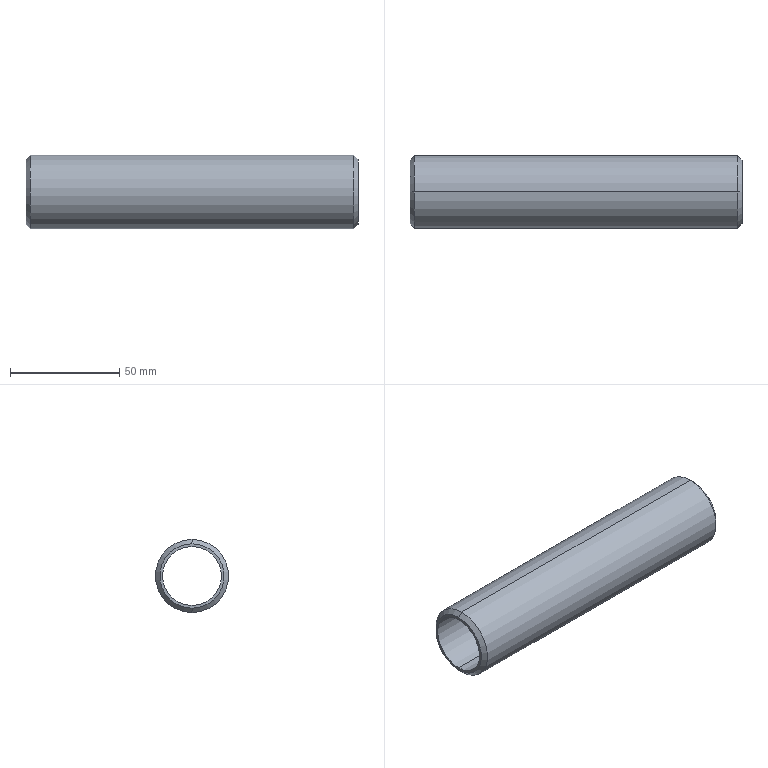Part | SolidWorks | features Chamfer 1, ExtruThin 1 | 1 solid | 10 faces | box 152 x 33.5 x 33.5 mm | volume 46542 mm3 | cone 4 | cylinder 4 | plane 2 | commonest cylinder face diameters 27 x2 33.5 x2
STEP:
#1=CARTESIAN_POINT('',(0.,0.,14.75));
#2=VERTEX_POINT('',#1);
#3=CARTESIAN_POINT('',(0.,0.,-14.75));
#4=VERTEX_POINT('',#3);
#5=CARTESIAN_POINT('',(0.,0.,0.));
#6=DIRECTION('',(-1.,0.,0.));
#7=DIRECTION('',(0.,0.,-1.));
#8=AXIS2_PLACEMENT_3D('',#5,#6,#7);
#9=CIRCLE('',#8,14.75);
#10=EDGE_CURVE('',#2,#4,#9,.T.);
#11=ORIENTED_EDGE('',*,*,#10,.F.);
#12=CARTESIAN_POINT('',(2.,0.,16.75));
#13=VERTEX_POINT('',#12);
#14=CARTESIAN_POINT('',(2.,0.,16.75));
#15=DIRECTION('',(0.7071,0.,0.7071));
#16=VECTOR('',#15,1000.);
#17=LINE('',#14,#16);
#18=EDGE_CURVE('',#2,#13,#17,.T.);
#19=ORIENTED_EDGE('',*,*,#18,.T.);
#20=CARTESIAN_POINT('',(2.,0.,-16.75));
#21=VERTEX_POINT('',#20);
#22=CARTESIAN_POINT('',(2.,0.,0.));
#23=DIRECTION('',(1.,0.,0.));
#24=DIRECTION('',(0.,0.,-1.));
#25=AXIS2_PLACEMENT_3D('',#22,#23,#24);
#26=CIRCLE('',#25,16.75);
#27=EDGE_CURVE('',#21,#13,#26,.T.);
#28=ORIENTED_EDGE('',*,*,#27,.F.);
#29=CARTESIAN_POINT('',(2.,0.,-16.75));
#30=DIRECTION('',(0.7071,0.,-0.7071));
#31=VECTOR('',#30,1000.);
#32=LINE('',#29,#31);
#33=EDGE_CURVE('',#4,#21,#32,.T.);
#34=ORIENTED_EDGE('',*,*,#33,.F.);
#35=EDGE_LOOP('',(#11,#19,#28,#34));
#36=FACE_OUTER_BOUND('',#35,.T.);
#37=CARTESIAN_POINT('',(2.,0.,0.));
#38=DIRECTION('',(1.,0.,0.));
#39=DIRECTION('',(0.,0.,-1.));
#40=AXIS2_PLACEMENT_3D('',#37,#38,#39);
#41=CONICAL_SURFACE('',#40,16.75,0.7854);
#42=ADVANCED_FACE('',(#36),#41,.T.);
#43=CARTESIAN_POINT('',(152.,0.,-14.75));
#44=VERTEX_POINT('',#43);
#45=CARTESIAN_POINT('',(152.,0.,14.75));
#46=VERTEX_POINT('',#45);
#47=CARTESIAN_POINT('',(152.,0.,0.));
#48=DIRECTION('',(1.,0.,0.));
#49=DIRECTION('',(0.,0.,-1.));
#50=AXIS2_PLACEMENT_3D('',#47,#48,#49);
#51=CIRCLE('',#50,14.75);
#52=EDGE_CURVE('',#44,#46,#51,.T.);
#53=ORIENTED_EDGE('',*,*,#52,.F.);
#54=CARTESIAN_POINT('',(150.,0.,-16.75));
#55=VERTEX_POINT('',#54);
#56=CARTESIAN_POINT('',(152.,0.,-14.75));
#57=DIRECTION('',(-0.7071,0.,-0.7071));
#58=VECTOR('',#57,1000.);
#59=LINE('',#56,#58);
#60=EDGE_CURVE('',#44,#55,#59,.T.);
#61=ORIENTED_EDGE('',*,*,#60,.T.);
#62=CARTESIAN_POINT('',(150.,0.,16.75));
#63=VERTEX_POINT('',#62);
#64=CARTESIAN_POINT('',(150.,0.,0.));
#65=DIRECTION('',(-1.,0.,0.));
#66=DIRECTION('',(0.,0.,-1.));
#67=AXIS2_PLACEMENT_3D('',#64,#65,#66);
#68=CIRCLE('',#67,16.75);
#69=EDGE_CURVE('',#63,#55,#68,.T.);
#70=ORIENTED_EDGE('',*,*,#69,.F.);
#71=CARTESIAN_POINT('',(152.,0.,14.75));
#72=DIRECTION('',(-0.7071,0.,0.7071));
#73=VECTOR('',#72,1000.);
#74=LINE('',#71,#73);
#75=EDGE_CURVE('',#46,#63,#74,.T.);
#76=ORIENTED_EDGE('',*,*,#75,.F.);
#77=EDGE_LOOP('',(#53,#61,#70,#76));
#78=FACE_OUTER_BOUND('',#77,.T.);
#79=CARTESIAN_POINT('',(152.,0.,0.));
#80=DIRECTION('',(-1.,0.,0.));
#81=DIRECTION('',(0.,0.,1.));
#82=AXIS2_PLACEMENT_3D('',#79,#80,#81);
#83=CONICAL_SURFACE('',#82,14.75,0.7854);
#84=ADVANCED_FACE('',(#78),#83,.T.);
#85=CARTESIAN_POINT('',(152.,0.,13.5));
#86=VERTEX_POINT('',#85);
#87=CARTESIAN_POINT('',(152.,0.,-13.5));
#88=VERTEX_POINT('',#87);
#89=CARTESIAN_POINT('',(152.,0.,0.));
#90=DIRECTION('',(1.,0.,0.));
#91=DIRECTION('',(0.,0.,-1.));
#92=AXIS2_PLACEMENT_3D('',#89,#90,#91);
#93=CIRCLE('',#92,13.5);
#94=EDGE_CURVE('',#86,#88,#93,.T.);
#95=ORIENTED_EDGE('',*,*,#94,.T.);
#96=CARTESIAN_POINT('',(0.,0.,-13.5));
#97=VERTEX_POINT('',#96);
#98=CARTESIAN_POINT('',(152.,0.,-13.5));
#99=DIRECTION('',(-1.,0.,0.));
#100=VECTOR('',#99,1000.);
#101=LINE('',#98,#100);
#102=EDGE_CURVE('',#88,#97,#101,.T.);
#103=ORIENTED_EDGE('',*,*,#102,.T.);
#104=CARTESIAN_POINT('',(0.,0.,13.5));
#105=VERTEX_POINT('',#104);
#106=CARTESIAN_POINT('',(0.,0.,0.));
#107=DIRECTION('',(1.,0.,0.));
#108=DIRECTION('',(0.,0.,-1.));
#109=AXIS2_PLACEMENT_3D('',#106,#107,#108);
#110=CIRCLE('',#109,13.5);
#111=EDGE_CURVE('',#105,#97,#110,.T.);
#112=ORIENTED_EDGE('',*,*,#111,.F.);
#113=CARTESIAN_POINT('',(152.,0.,13.5));
#114=DIRECTION('',(-1.,0.,0.));
#115=VECTOR('',#114,1000.);
#116=LINE('',#113,#115);
#117=EDGE_CURVE('',#86,#105,#116,.T.);
#118=ORIENTED_EDGE('',*,*,#117,.F.);
#119=EDGE_LOOP('',(#95,#103,#112,#118));
#120=FACE_OUTER_BOUND('',#119,.T.);
#121=CARTESIAN_POINT('',(152.,0.,0.));
#122=DIRECTION('',(-1.,0.,0.));
#123=DIRECTION('',(0.,0.,1.));
#124=AXIS2_PLACEMENT_3D('',#121,#122,#123);
#125=CYLINDRICAL_SURFACE('',#124,13.5);
#126=ADVANCED_FACE('',(#120),#125,.F.);
#127=ORIENTED_EDGE('',*,*,#69,.T.);
#128=CARTESIAN_POINT('',(152.,0.,-16.75));
#129=DIRECTION('',(-1.,0.,0.));
#130=VECTOR('',#129,1000.);
#131=LINE('',#128,#130);
#132=EDGE_CURVE('',#55,#21,#131,.T.);
#133=ORIENTED_EDGE('',*,*,#132,.T.);
#134=ORIENTED_EDGE('',*,*,#27,.T.);
#135=CARTESIAN_POINT('',(152.,0.,16.75));
#136=DIRECTION('',(-1.,0.,0.));
#137=VECTOR('',#136,1000.);
#138=LINE('',#135,#137);
#139=EDGE_CURVE('',#63,#13,#138,.T.);
#140=ORIENTED_EDGE('',*,*,#139,.F.);
#141=EDGE_LOOP('',(#127,#133,#134,#140));
#142=FACE_OUTER_BOUND('',#141,.T.);
#143=CARTESIAN_POINT('',(152.,0.,0.));
#144=DIRECTION('',(-1.,0.,0.));
#145=DIRECTION('',(0.,0.,1.));
#146=AXIS2_PLACEMENT_3D('',#143,#144,#145);
#147=CYLINDRICAL_SURFACE('',#146,16.75);
#148=ADVANCED_FACE('',(#142),#147,.T.);
#149=CARTESIAN_POINT('',(152.,0.,0.));
#150=DIRECTION('',(1.,0.,0.));
#151=DIRECTION('',(0.,0.,-1.));
#152=AXIS2_PLACEMENT_3D('',#149,#150,#151);
#153=CIRCLE('',#152,14.75);
#154=EDGE_CURVE('',#46,#44,#153,.T.);
#155=ORIENTED_EDGE('',*,*,#154,.T.);
#156=ORIENTED_EDGE('',*,*,#52,.T.);
#157=EDGE_LOOP('',(#155,#156));
#158=FACE_OUTER_BOUND('',#157,.T.);
#159=ORIENTED_EDGE('',*,*,#94,.F.);
#160=CARTESIAN_POINT('',(152.,0.,0.));
#161=DIRECTION('',(1.,0.,0.));
#162=DIRECTION('',(0.,0.,-1.));
#163=AXIS2_PLACEMENT_3D('',#160,#161,#162);
#164=CIRCLE('',#163,13.5);
#165=EDGE_CURVE('',#88,#86,#164,.T.);
#166=ORIENTED_EDGE('',*,*,#165,.F.);
#167=EDGE_LOOP('',(#159,#166));
#168=FACE_BOUND('',#167,.T.);
#169=CARTESIAN_POINT('',(152.,0.,0.));
#170=DIRECTION('',(1.,0.,0.));
#171=DIRECTION('',(0.,0.,-1.));
#172=AXIS2_PLACEMENT_3D('',#169,#170,#171);
#173=PLANE('',#172);
#174=ADVANCED_FACE('',(#158,#168),#173,.T.);
#175=CARTESIAN_POINT('',(0.,0.,0.));
#176=DIRECTION('',(-1.,0.,0.));
#177=DIRECTION('',(0.,0.,-1.));
#178=AXIS2_PLACEMENT_3D('',#175,#176,#177);
#179=CIRCLE('',#178,14.75);
#180=EDGE_CURVE('',#4,#2,#179,.T.);
#181=ORIENTED_EDGE('',*,*,#180,.T.);
#182=ORIENTED_EDGE('',*,*,#10,.T.);
#183=EDGE_LOOP('',(#181,#182));
#184=FACE_OUTER_BOUND('',#183,.T.);
#185=ORIENTED_EDGE('',*,*,#111,.T.);
#186=CARTESIAN_POINT('',(0.,0.,0.));
#187=DIRECTION('',(1.,0.,0.));
#188=DIRECTION('',(0.,0.,-1.));
#189=AXIS2_PLACEMENT_3D('',#186,#187,#188);
#190=CIRCLE('',#189,13.5);
#191=EDGE_CURVE('',#97,#105,#190,.T.);
#192=ORIENTED_EDGE('',*,*,#191,.T.);
#193=EDGE_LOOP('',(#185,#192));
#194=FACE_BOUND('',#193,.T.);
#195=CARTESIAN_POINT('',(0.,0.,0.));
#196=DIRECTION('',(1.,0.,0.));
#197=DIRECTION('',(0.,0.,-1.));
#198=AXIS2_PLACEMENT_3D('',#195,#196,#197);
#199=PLANE('',#198);
#200=ADVANCED_FACE('',(#184,#194),#199,.F.);
#201=ORIENTED_EDGE('',*,*,#132,.F.);
#202=CARTESIAN_POINT('',(150.,0.,0.));
#203=DIRECTION('',(-1.,0.,0.));
#204=DIRECTION('',(0.,0.,-1.));
#205=AXIS2_PLACEMENT_3D('',#202,#203,#204);
#206=CIRCLE('',#205,16.75);
#207=EDGE_CURVE('',#55,#63,#206,.T.);
#208=ORIENTED_EDGE('',*,*,#207,.T.);
#209=ORIENTED_EDGE('',*,*,#139,.T.);
#210=CARTESIAN_POINT('',(2.,0.,0.));
#211=DIRECTION('',(1.,0.,0.));
#212=DIRECTION('',(0.,0.,-1.));
#213=AXIS2_PLACEMENT_3D('',#210,#211,#212);
#214=CIRCLE('',#213,16.75);
#215=EDGE_CURVE('',#13,#21,#214,.T.);
#216=ORIENTED_EDGE('',*,*,#215,.T.);
#217=EDGE_LOOP('',(#201,#208,#209,#216));
#218=FACE_OUTER_BOUND('',#217,.T.);
#219=CARTESIAN_POINT('',(152.,0.,0.));
#220=DIRECTION('',(-1.,0.,0.));
#221=DIRECTION('',(0.,0.,1.));
#222=AXIS2_PLACEMENT_3D('',#219,#220,#221);
#223=CYLINDRICAL_SURFACE('',#222,16.75);
#224=ADVANCED_FACE('',(#218),#223,.T.);
#225=ORIENTED_EDGE('',*,*,#102,.F.);
#226=ORIENTED_EDGE('',*,*,#165,.T.);
#227=ORIENTED_EDGE('',*,*,#117,.T.);
#228=ORIENTED_EDGE('',*,*,#191,.F.);
#229=EDGE_LOOP('',(#225,#226,#227,#228));
#230=FACE_OUTER_BOUND('',#229,.T.);
#231=CARTESIAN_POINT('',(152.,0.,0.));
#232=DIRECTION('',(-1.,0.,0.));
#233=DIRECTION('',(0.,0.,1.));
#234=AXIS2_PLACEMENT_3D('',#231,#232,#233);
#235=CYLINDRICAL_SURFACE('',#234,13.5);
#236=ADVANCED_FACE('',(#230),#235,.F.);
#237=ORIENTED_EDGE('',*,*,#60,.F.);
#238=ORIENTED_EDGE('',*,*,#154,.F.);
#239=ORIENTED_EDGE('',*,*,#75,.T.);
#240=ORIENTED_EDGE('',*,*,#207,.F.);
#241=EDGE_LOOP('',(#237,#238,#239,#240));
#242=FACE_OUTER_BOUND('',#241,.T.);
#243=CARTESIAN_POINT('',(152.,0.,0.));
#244=DIRECTION('',(-1.,0.,0.));
#245=DIRECTION('',(0.,0.,1.));
#246=AXIS2_PLACEMENT_3D('',#243,#244,#245);
#247=CONICAL_SURFACE('',#246,14.75,0.7854);
#248=ADVANCED_FACE('',(#242),#247,.T.);
#249=ORIENTED_EDGE('',*,*,#18,.F.);
#250=ORIENTED_EDGE('',*,*,#180,.F.);
#251=ORIENTED_EDGE('',*,*,#33,.T.);
#252=ORIENTED_EDGE('',*,*,#215,.F.);
#253=EDGE_LOOP('',(#249,#250,#251,#252));
#254=FACE_OUTER_BOUND('',#253,.T.);
#255=CARTESIAN_POINT('',(2.,0.,0.));
#256=DIRECTION('',(1.,0.,0.));
#257=DIRECTION('',(0.,0.,-1.));
#258=AXIS2_PLACEMENT_3D('',#255,#256,#257);
#259=CONICAL_SURFACE('',#258,16.75,0.7854);
#260=ADVANCED_FACE('',(#254),#259,.T.);
#261=CLOSED_SHELL('',(#42,#84,#126,#148,#174,#200,#224,#236,#248,#260));
#262=MANIFOLD_SOLID_BREP('',#261);
#263=CARTESIAN_POINT('',(0.,0.,0.));
#264=DIRECTION('',(0.,0.,1.));
#265=DIRECTION('',(1.,0.,0.));
#266=AXIS2_PLACEMENT_3D('',#263,#264,#265);
#267=(LENGTH_UNIT()NAMED_UNIT(*)SI_UNIT(.MILLI.,.METRE.));
#268=UNCERTAINTY_MEASURE_WITH_UNIT(LENGTH_MEASURE(0.00001),#267,'','');
#269=(NAMED_UNIT(*)PLANE_ANGLE_UNIT()SI_UNIT($,.RADIAN.));
#270=(NAMED_UNIT(*)SI_UNIT($,.STERADIAN.)SOLID_ANGLE_UNIT());
#271=(GEOMETRIC_REPRESENTATION_CONTEXT(3)GLOBAL_UNCERTAINTY_ASSIGNED_CONTEXT((#268))GLOBAL_UNIT_ASSIGNED_CONTEXT((#267,#269,#270))REPRESENTATION_CONTEXT('',''));
#272=ADVANCED_BREP_SHAPE_REPRESENTATION('',(#262,#266),#271);